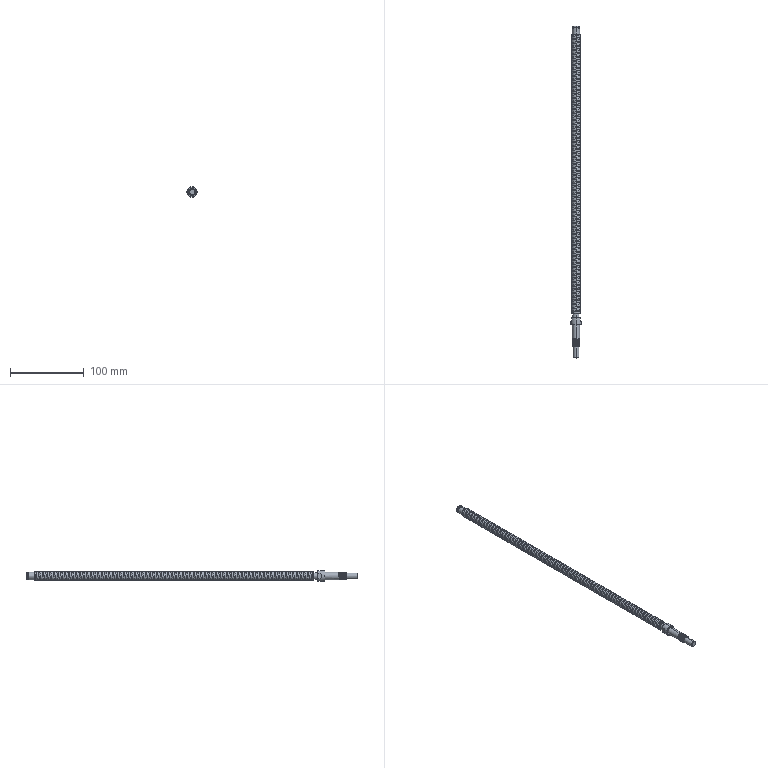Part | NX | features BREP 1 | 1 solid | 225 faces | box 14 x 451.1 x 14 mm | volume 44527 mm3 | cylinder 189 | cone 17 | plane 16 | spline 3 | commonest cylinder face diameters 12 x153 10 x26 9.5 x4 8 x3 14 x2 8.917 x1